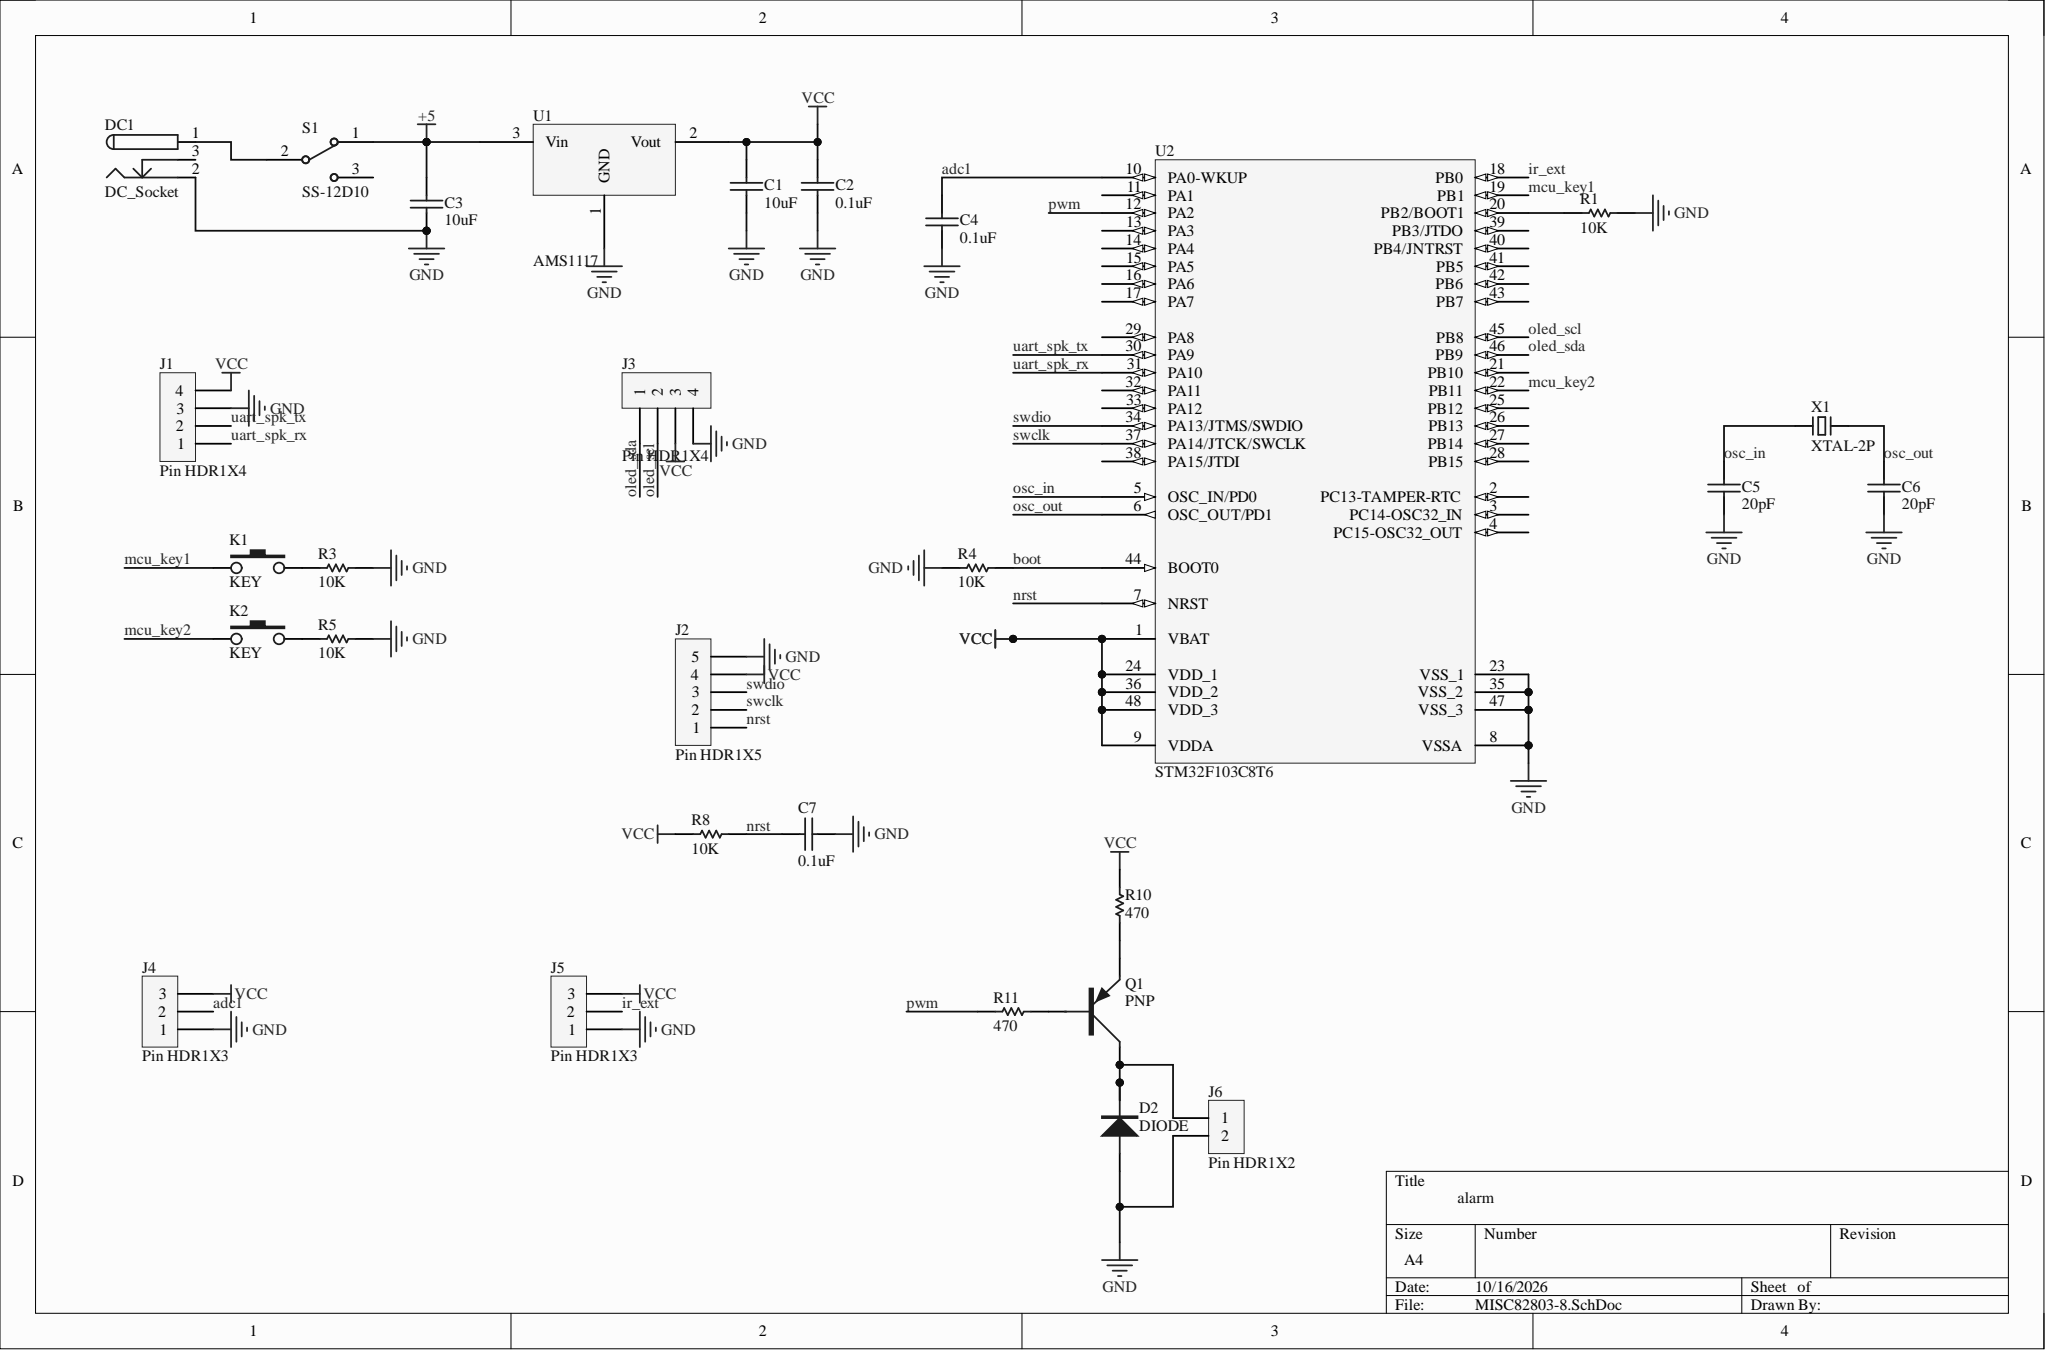Circuit board | Altium Designer | 29 parts | 25 nets
Bill of materials:
Comment,Description,Designator,Footprint,LibRef,Quantity
"10uF","Non-polar capacitor","C1, C3","0603C","CAP","2"
"0.1uF","Non-polar capacitor","C2, C4, C7","0603C","CAP","3"
"20pF","Non-polar capacitor","C5, C6","0603C","CAP","2"
"DIODE","General diode","D2","SOD-123","DIODE","1"
"DC_Socket","","DC1","DC-002","DC_Socket","1"
"Pin HDR1X4","","J1, J3","Pin HDR1X4/2.54mm-S","Pin HDR1X4","2"
"Pin HDR1X5","","J2","Pin HDR1X5/2.54mm-S","Pin HDR1X5","1"
"Pin HDR1X3","","J4, J5","Pin HDR1X3/2.54mm-S","Pin HDR1X3","2"
"Pin HDR1X2","","J6","Pin HDR1X2/2.54mm-S","Pin HDR1X2","1"
"KEY","","K1, K2","DIP-3X6X4.3","KEY","2"
"PNP","PNP transistor","Q1","SOT-23","PNP","1"
"10K","","R1, R3, R4, R5, R8","0603R","RES","5"
"470","","R10, R11","0603R","RES","2"
"SS-12D10","","S1","SS-12D10","SS-12D10","1"
"AMS1117","Three-terminal voltage regulator","U1","SOT223","AMS1117","1"
"STM32F103C8T6","","U2","LQFP48 7X7","STM32F103C8T6","1"
"XTAL-2P","2-pin passive crystal oscillator","X1","OSC HC-49S","XTAL-2P","1"
Netlist (Protel format):
[
C1
0603C
10uF



]
[
C2
0603C
0.1uF



]
[
C3
0603C
10uF



]
[
C4
0603C
0.1uF



]
[
C5
0603C
20pF



]
[
C6
0603C
20pF



]
[
C7
0603C
0.1uF



]
[
D2
SOD-123
DIODE



]
[
DC1
DC-002
DC_Socket



]
[
J1
Pin HDR1X4/2.54mm-S
Pin HDR1X4



]
[
J2
Pin HDR1X5/2.54mm-S
Pin HDR1X5



]
[
J3
Pin HDR1X4/2.54mm-S
Pin HDR1X4



]
[
J4
Pin HDR1X3/2.54mm-S
Pin HDR1X3



]
[
J5
Pin HDR1X3/2.54mm-S
Pin HDR1X3



]
[
J6
Pin HDR1X2/2.54mm-S
Pin HDR1X2



]
[
K1
DIP-3X6X4.3
KEY



]
[
K2
DIP-3X6X4.3
KEY



]
[
Q1
SOT-23
PNP



]
[
R1
0603R
10K



]
[
R3
0603R
10K



]
[
R4
0603R
10K



]
[
R5
0603R
10K



]
[
R8
0603R
10K



]
[
R10
0603R
470



]
[
R11
0603R
470



]
[
S1
SS-12D10
SS-12D10



]
[
U1
SOT223
AMS1117



]
[
U2
LQFP48 7X7
STM32F103C8T6



]
[
X1
OSC HC-49S
XTAL-2P



]
(
VCC
C1-2
C2-2
J1-4
J2-4
J3-3
J4-3
J5-3
R8-2
R10-1
U1-2
U2-1
U2-9
U2-24
U2-36
U2-48
)
(
uart_spk_tx
J1-2
U2-30
)
(
uart_spk_rx
J1-1
U2-31
)
(
swdio
J2-3
U2-34
)
(
swclk
J2-2
U2-37
)
(
pwm
R11-1
U2-12
)
(
osc_out
C6-2
U2-6
X1-2
)
(
osc_in
C5-2
U2-5
X1-1
)
(
oled_sda
J3-1
U2-46
)
(
oled_scl
J3-2
U2-45
)
(
nrst
C7-2
J2-1
R8-1
U2-7
)
(
NetR1_2
R1-2
U2-20
)
(
NetQ1_E
Q1-E
R10-2
)
(
NetQ1_B
Q1-B
R11-2
)
(
NetK2_3
K2-3
R5-2
)
(
NetK1_3
K1-3
R3-2
)
(
NetDC1_1
DC1-1
S1-2
)
(
NetD2_K
D2-K
J6-1
Q1-C
)
(
mcu_key2
K2-1
U2-22
)
(
mcu_key1
K1-1
U2-19
)
(
ir_ext
J5-2
U2-18
)
(
GND
C1-1
C2-1
C3-1
C4-1
C5-1
C6-1
C7-1
D2-A
DC1-2
J1-3
J2-5
J3-4
J4-1
J5-1
J6-2
R1-1
R3-1
R4-2
R5-1
U1-1
U2-8
U2-23
U2-35
U2-47
)
(
boot
R4-1
U2-44
)
(
adc1
C4-2
J4-2
U2-10
)
(
+5
C3-2
S1-1
U1-3
)